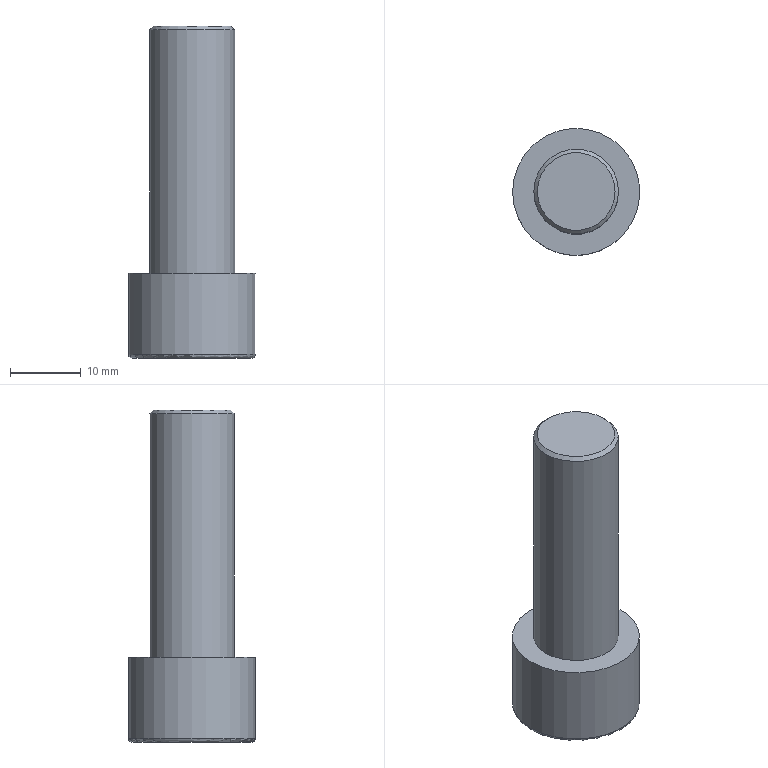Part | NX | features solid 2 | 1 solid | 14 faces | box 18 x 18 x 47 mm | volume 6485 mm3 | plane 10 | cylinder 2 | torus 1 | cone 1 | commonest cylinder face diameters 12 x1 18 x1
STEP:
#1=CARTESIAN_POINT('',(-119.887,-217.,-374.5));
#2=VERTEX_POINT('',#1);
#3=CARTESIAN_POINT('',(-122.774,-212.,-374.5));
#4=VERTEX_POINT('',#3);
#5=CARTESIAN_POINT('',(-119.887,-217.,-374.5));
#6=DIRECTION('',(-0.5,0.866,0.));
#7=VECTOR('',#6,1000.);
#8=LINE('',#5,#7);
#9=EDGE_CURVE('',#2,#4,#8,.T.);
#10=ORIENTED_EDGE('',*,*,#9,.F.);
#11=CARTESIAN_POINT('',(-114.113,-217.,-374.5));
#12=VERTEX_POINT('',#11);
#13=CARTESIAN_POINT('',(-114.113,-217.,-374.5));
#14=DIRECTION('',(-1.,0.,0.));
#15=VECTOR('',#14,1000.);
#16=LINE('',#13,#15);
#17=EDGE_CURVE('',#12,#2,#16,.T.);
#18=ORIENTED_EDGE('',*,*,#17,.F.);
#19=CARTESIAN_POINT('',(-111.226,-212.,-374.5));
#20=VERTEX_POINT('',#19);
#21=CARTESIAN_POINT('',(-111.226,-212.,-374.5));
#22=DIRECTION('',(-0.5,-0.866,0.));
#23=VECTOR('',#22,1000.);
#24=LINE('',#21,#23);
#25=EDGE_CURVE('',#20,#12,#24,.T.);
#26=ORIENTED_EDGE('',*,*,#25,.F.);
#27=CARTESIAN_POINT('',(-114.113,-207.,-374.5));
#28=VERTEX_POINT('',#27);
#29=CARTESIAN_POINT('',(-114.113,-207.,-374.5));
#30=DIRECTION('',(0.5,-0.866,0.));
#31=VECTOR('',#30,1000.);
#32=LINE('',#29,#31);
#33=EDGE_CURVE('',#28,#20,#32,.T.);
#34=ORIENTED_EDGE('',*,*,#33,.F.);
#35=CARTESIAN_POINT('',(-119.887,-207.,-374.5));
#36=VERTEX_POINT('',#35);
#37=CARTESIAN_POINT('',(-119.887,-207.,-374.5));
#38=DIRECTION('',(1.,0.,0.));
#39=VECTOR('',#38,1000.);
#40=LINE('',#37,#39);
#41=EDGE_CURVE('',#36,#28,#40,.T.);
#42=ORIENTED_EDGE('',*,*,#41,.F.);
#43=CARTESIAN_POINT('',(-122.774,-212.,-374.5));
#44=DIRECTION('',(0.5,0.866,0.));
#45=VECTOR('',#44,1000.);
#46=LINE('',#43,#45);
#47=EDGE_CURVE('',#4,#36,#46,.T.);
#48=ORIENTED_EDGE('',*,*,#47,.F.);
#49=EDGE_LOOP('',(#10,#18,#26,#34,#42,#48));
#50=FACE_BOUND('',#49,.T.);
#51=CARTESIAN_POINT('',(-125.5,-212.,-374.5));
#52=VERTEX_POINT('',#51);
#53=CARTESIAN_POINT('',(-117.,-212.,-374.5));
#54=DIRECTION('',(0.,0.,-1.));
#55=DIRECTION('',(-1.,0.,0.));
#56=AXIS2_PLACEMENT_3D('',#53,#54,#55);
#57=CIRCLE('',#56,8.5);
#58=EDGE_CURVE('',#52,#52,#57,.T.);
#59=ORIENTED_EDGE('',*,*,#58,.T.);
#60=EDGE_LOOP('',(#59));
#61=FACE_BOUND('',#60,.T.);
#62=CARTESIAN_POINT('',(-117.,-212.,-374.5));
#63=DIRECTION('',(0.,0.,-1.));
#64=DIRECTION('',(-1.,0.,0.));
#65=AXIS2_PLACEMENT_3D('',#62,#63,#64);
#66=PLANE('',#65);
#67=ADVANCED_FACE('',(#50,#61),#66,.T.);
#68=CARTESIAN_POINT('',(-111.,-212.,-362.5));
#69=VERTEX_POINT('',#68);
#70=CARTESIAN_POINT('',(-117.,-212.,-362.5));
#71=DIRECTION('',(0.,0.,1.));
#72=DIRECTION('',(1.,0.,0.));
#73=AXIS2_PLACEMENT_3D('',#70,#71,#72);
#74=CIRCLE('',#73,6.);
#75=EDGE_CURVE('',#69,#69,#74,.T.);
#76=ORIENTED_EDGE('',*,*,#75,.F.);
#77=EDGE_LOOP('',(#76));
#78=FACE_BOUND('',#77,.T.);
#79=CARTESIAN_POINT('',(-126.,-212.,-362.5));
#80=VERTEX_POINT('',#79);
#81=CARTESIAN_POINT('',(-117.,-212.,-362.5));
#82=DIRECTION('',(0.,0.,-1.));
#83=DIRECTION('',(-1.,0.,0.));
#84=AXIS2_PLACEMENT_3D('',#81,#82,#83);
#85=CIRCLE('',#84,9.);
#86=EDGE_CURVE('',#80,#80,#85,.T.);
#87=ORIENTED_EDGE('',*,*,#86,.F.);
#88=EDGE_LOOP('',(#87));
#89=FACE_BOUND('',#88,.T.);
#90=CARTESIAN_POINT('',(-117.,-212.,-362.5));
#91=DIRECTION('',(0.,0.,1.));
#92=DIRECTION('',(1.,0.,0.));
#93=AXIS2_PLACEMENT_3D('',#90,#91,#92);
#94=PLANE('',#93);
#95=ADVANCED_FACE('',(#78,#89),#94,.T.);
#96=CARTESIAN_POINT('',(-126.,-212.,-374.));
#97=VERTEX_POINT('',#96);
#98=CARTESIAN_POINT('',(-117.,-212.,-374.));
#99=DIRECTION('',(0.,0.,-1.));
#100=DIRECTION('',(-1.,0.,0.));
#101=AXIS2_PLACEMENT_3D('',#98,#99,#100);
#102=CIRCLE('',#101,9.);
#103=EDGE_CURVE('',#97,#97,#102,.F.);
#104=ORIENTED_EDGE('',*,*,#103,.T.);
#105=EDGE_LOOP('',(#104));
#106=FACE_BOUND('',#105,.T.);
#107=ORIENTED_EDGE('',*,*,#86,.T.);
#108=EDGE_LOOP('',(#107));
#109=FACE_BOUND('',#108,.T.);
#110=CARTESIAN_POINT('',(-117.,-212.,-362.5));
#111=DIRECTION('',(0.,0.,-1.));
#112=DIRECTION('',(-1.,0.,0.));
#113=AXIS2_PLACEMENT_3D('',#110,#111,#112);
#114=CYLINDRICAL_SURFACE('',#113,9.);
#115=ADVANCED_FACE('',(#106,#109),#114,.T.);
#116=ORIENTED_EDGE('',*,*,#58,.F.);
#117=EDGE_LOOP('',(#116));
#118=FACE_BOUND('',#117,.T.);
#119=ORIENTED_EDGE('',*,*,#103,.F.);
#120=EDGE_LOOP('',(#119));
#121=FACE_BOUND('',#120,.T.);
#122=CARTESIAN_POINT('',(-117.,-212.,-374.));
#123=DIRECTION('',(0.,0.,-1.));
#124=DIRECTION('',(-1.,0.,0.));
#125=AXIS2_PLACEMENT_3D('',#122,#123,#124);
#126=TOROIDAL_SURFACE('',#125,8.5,0.5);
#127=ADVANCED_FACE('',(#118,#121),#126,.T.);
#128=CARTESIAN_POINT('',(-111.5,-212.,-327.5));
#129=VERTEX_POINT('',#128);
#130=CARTESIAN_POINT('',(-117.,-212.,-327.5));
#131=DIRECTION('',(0.,0.,1.));
#132=DIRECTION('',(1.,0.,0.));
#133=AXIS2_PLACEMENT_3D('',#130,#131,#132);
#134=CIRCLE('',#133,5.5);
#135=EDGE_CURVE('',#129,#129,#134,.T.);
#136=ORIENTED_EDGE('',*,*,#135,.T.);
#137=EDGE_LOOP('',(#136));
#138=FACE_BOUND('',#137,.T.);
#139=CARTESIAN_POINT('',(-117.,-212.,-327.5));
#140=DIRECTION('',(0.,0.,1.));
#141=DIRECTION('',(1.,0.,0.));
#142=AXIS2_PLACEMENT_3D('',#139,#140,#141);
#143=PLANE('',#142);
#144=ADVANCED_FACE('',(#138),#143,.T.);
#145=CARTESIAN_POINT('',(-111.,-212.,-328.));
#146=VERTEX_POINT('',#145);
#147=CARTESIAN_POINT('',(-117.,-212.,-328.));
#148=DIRECTION('',(0.,0.,1.));
#149=DIRECTION('',(1.,0.,0.));
#150=AXIS2_PLACEMENT_3D('',#147,#148,#149);
#151=CIRCLE('',#150,6.);
#152=EDGE_CURVE('',#146,#146,#151,.F.);
#153=ORIENTED_EDGE('',*,*,#152,.T.);
#154=EDGE_LOOP('',(#153));
#155=FACE_BOUND('',#154,.T.);
#156=ORIENTED_EDGE('',*,*,#75,.T.);
#157=EDGE_LOOP('',(#156));
#158=FACE_BOUND('',#157,.T.);
#159=CARTESIAN_POINT('',(-117.,-212.,-327.5));
#160=DIRECTION('',(0.,0.,-1.));
#161=DIRECTION('',(-1.,0.,0.));
#162=AXIS2_PLACEMENT_3D('',#159,#160,#161);
#163=CYLINDRICAL_SURFACE('',#162,6.);
#164=ADVANCED_FACE('',(#155,#158),#163,.T.);
#165=ORIENTED_EDGE('',*,*,#135,.F.);
#166=EDGE_LOOP('',(#165));
#167=FACE_BOUND('',#166,.T.);
#168=ORIENTED_EDGE('',*,*,#152,.F.);
#169=EDGE_LOOP('',(#168));
#170=FACE_BOUND('',#169,.T.);
#171=CARTESIAN_POINT('',(-117.,-212.,-328.));
#172=DIRECTION('',(0.,0.,-1.));
#173=DIRECTION('',(-1.,0.,0.));
#174=AXIS2_PLACEMENT_3D('',#171,#172,#173);
#175=CONICAL_SURFACE('',#174,6.,0.7854);
#176=ADVANCED_FACE('',(#167,#170),#175,.T.);
#177=ORIENTED_EDGE('',*,*,#9,.T.);
#178=CARTESIAN_POINT('',(-122.774,-212.,-368.5));
#179=VERTEX_POINT('',#178);
#180=CARTESIAN_POINT('',(-122.774,-212.,-368.5));
#181=DIRECTION('',(0.,0.,-1.));
#182=VECTOR('',#181,1000.);
#183=LINE('',#180,#182);
#184=EDGE_CURVE('',#179,#4,#183,.T.);
#185=ORIENTED_EDGE('',*,*,#184,.F.);
#186=CARTESIAN_POINT('',(-119.887,-217.,-368.5));
#187=VERTEX_POINT('',#186);
#188=CARTESIAN_POINT('',(-119.887,-217.,-368.5));
#189=DIRECTION('',(-0.5,0.866,0.));
#190=VECTOR('',#189,1000.);
#191=LINE('',#188,#190);
#192=EDGE_CURVE('',#187,#179,#191,.T.);
#193=ORIENTED_EDGE('',*,*,#192,.F.);
#194=CARTESIAN_POINT('',(-119.887,-217.,-368.5));
#195=DIRECTION('',(0.,0.,-1.));
#196=VECTOR('',#195,1000.);
#197=LINE('',#194,#196);
#198=EDGE_CURVE('',#187,#2,#197,.T.);
#199=ORIENTED_EDGE('',*,*,#198,.T.);
#200=EDGE_LOOP('',(#177,#185,#193,#199));
#201=FACE_BOUND('',#200,.T.);
#202=CARTESIAN_POINT('',(-121.33,-214.5,-371.5));
#203=DIRECTION('',(-0.866,-0.5,0.));
#204=DIRECTION('',(0.5,-0.866,0.));
#205=AXIS2_PLACEMENT_3D('',#202,#203,#204);
#206=PLANE('',#205);
#207=ADVANCED_FACE('',(#201),#206,.F.);
#208=ORIENTED_EDGE('',*,*,#17,.T.);
#209=ORIENTED_EDGE('',*,*,#198,.F.);
#210=CARTESIAN_POINT('',(-114.113,-217.,-368.5));
#211=VERTEX_POINT('',#210);
#212=CARTESIAN_POINT('',(-114.113,-217.,-368.5));
#213=DIRECTION('',(-1.,0.,0.));
#214=VECTOR('',#213,1000.);
#215=LINE('',#212,#214);
#216=EDGE_CURVE('',#211,#187,#215,.T.);
#217=ORIENTED_EDGE('',*,*,#216,.F.);
#218=CARTESIAN_POINT('',(-114.113,-217.,-368.5));
#219=DIRECTION('',(0.,0.,-1.));
#220=VECTOR('',#219,1000.);
#221=LINE('',#218,#220);
#222=EDGE_CURVE('',#211,#12,#221,.T.);
#223=ORIENTED_EDGE('',*,*,#222,.T.);
#224=EDGE_LOOP('',(#208,#209,#217,#223));
#225=FACE_BOUND('',#224,.T.);
#226=CARTESIAN_POINT('',(-117.,-217.,-371.5));
#227=DIRECTION('',(0.,-1.,0.));
#228=DIRECTION('',(1.,0.,0.));
#229=AXIS2_PLACEMENT_3D('',#226,#227,#228);
#230=PLANE('',#229);
#231=ADVANCED_FACE('',(#225),#230,.F.);
#232=ORIENTED_EDGE('',*,*,#25,.T.);
#233=ORIENTED_EDGE('',*,*,#222,.F.);
#234=CARTESIAN_POINT('',(-111.226,-212.,-368.5));
#235=VERTEX_POINT('',#234);
#236=CARTESIAN_POINT('',(-111.226,-212.,-368.5));
#237=DIRECTION('',(-0.5,-0.866,0.));
#238=VECTOR('',#237,1000.);
#239=LINE('',#236,#238);
#240=EDGE_CURVE('',#235,#211,#239,.T.);
#241=ORIENTED_EDGE('',*,*,#240,.F.);
#242=CARTESIAN_POINT('',(-111.226,-212.,-368.5));
#243=DIRECTION('',(0.,0.,-1.));
#244=VECTOR('',#243,1000.);
#245=LINE('',#242,#244);
#246=EDGE_CURVE('',#235,#20,#245,.T.);
#247=ORIENTED_EDGE('',*,*,#246,.T.);
#248=EDGE_LOOP('',(#232,#233,#241,#247));
#249=FACE_BOUND('',#248,.T.);
#250=CARTESIAN_POINT('',(-112.67,-214.5,-371.5));
#251=DIRECTION('',(0.866,-0.5,0.));
#252=DIRECTION('',(0.5,0.866,0.));
#253=AXIS2_PLACEMENT_3D('',#250,#251,#252);
#254=PLANE('',#253);
#255=ADVANCED_FACE('',(#249),#254,.F.);
#256=ORIENTED_EDGE('',*,*,#33,.T.);
#257=ORIENTED_EDGE('',*,*,#246,.F.);
#258=CARTESIAN_POINT('',(-114.113,-207.,-368.5));
#259=VERTEX_POINT('',#258);
#260=CARTESIAN_POINT('',(-114.113,-207.,-368.5));
#261=DIRECTION('',(0.5,-0.866,0.));
#262=VECTOR('',#261,1000.);
#263=LINE('',#260,#262);
#264=EDGE_CURVE('',#259,#235,#263,.T.);
#265=ORIENTED_EDGE('',*,*,#264,.F.);
#266=CARTESIAN_POINT('',(-114.113,-207.,-368.5));
#267=DIRECTION('',(0.,0.,-1.));
#268=VECTOR('',#267,1000.);
#269=LINE('',#266,#268);
#270=EDGE_CURVE('',#259,#28,#269,.T.);
#271=ORIENTED_EDGE('',*,*,#270,.T.);
#272=EDGE_LOOP('',(#256,#257,#265,#271));
#273=FACE_BOUND('',#272,.T.);
#274=CARTESIAN_POINT('',(-112.67,-209.5,-371.5));
#275=DIRECTION('',(0.866,0.5,0.));
#276=DIRECTION('',(-0.5,0.866,0.));
#277=AXIS2_PLACEMENT_3D('',#274,#275,#276);
#278=PLANE('',#277);
#279=ADVANCED_FACE('',(#273),#278,.F.);
#280=ORIENTED_EDGE('',*,*,#41,.T.);
#281=ORIENTED_EDGE('',*,*,#270,.F.);
#282=CARTESIAN_POINT('',(-119.887,-207.,-368.5));
#283=VERTEX_POINT('',#282);
#284=CARTESIAN_POINT('',(-119.887,-207.,-368.5));
#285=DIRECTION('',(1.,0.,0.));
#286=VECTOR('',#285,1000.);
#287=LINE('',#284,#286);
#288=EDGE_CURVE('',#283,#259,#287,.T.);
#289=ORIENTED_EDGE('',*,*,#288,.F.);
#290=CARTESIAN_POINT('',(-119.887,-207.,-368.5));
#291=DIRECTION('',(0.,0.,-1.));
#292=VECTOR('',#291,1000.);
#293=LINE('',#290,#292);
#294=EDGE_CURVE('',#283,#36,#293,.T.);
#295=ORIENTED_EDGE('',*,*,#294,.T.);
#296=EDGE_LOOP('',(#280,#281,#289,#295));
#297=FACE_BOUND('',#296,.T.);
#298=CARTESIAN_POINT('',(-117.,-207.,-371.5));
#299=DIRECTION('',(0.,1.,0.));
#300=DIRECTION('',(0.,0.,1.));
#301=AXIS2_PLACEMENT_3D('',#298,#299,#300);
#302=PLANE('',#301);
#303=ADVANCED_FACE('',(#297),#302,.F.);
#304=ORIENTED_EDGE('',*,*,#47,.T.);
#305=ORIENTED_EDGE('',*,*,#294,.F.);
#306=CARTESIAN_POINT('',(-122.774,-212.,-368.5));
#307=DIRECTION('',(0.5,0.866,0.));
#308=VECTOR('',#307,1000.);
#309=LINE('',#306,#308);
#310=EDGE_CURVE('',#179,#283,#309,.T.);
#311=ORIENTED_EDGE('',*,*,#310,.F.);
#312=ORIENTED_EDGE('',*,*,#184,.T.);
#313=EDGE_LOOP('',(#304,#305,#311,#312));
#314=FACE_BOUND('',#313,.T.);
#315=CARTESIAN_POINT('',(-121.33,-209.5,-371.5));
#316=DIRECTION('',(-0.866,0.5,0.));
#317=DIRECTION('',(-0.5,-0.866,0.));
#318=AXIS2_PLACEMENT_3D('',#315,#316,#317);
#319=PLANE('',#318);
#320=ADVANCED_FACE('',(#314),#319,.F.);
#321=ORIENTED_EDGE('',*,*,#310,.T.);
#322=ORIENTED_EDGE('',*,*,#288,.T.);
#323=ORIENTED_EDGE('',*,*,#264,.T.);
#324=ORIENTED_EDGE('',*,*,#240,.T.);
#325=ORIENTED_EDGE('',*,*,#216,.T.);
#326=ORIENTED_EDGE('',*,*,#192,.T.);
#327=EDGE_LOOP('',(#321,#322,#323,#324,#325,#326));
#328=FACE_BOUND('',#327,.T.);
#329=CARTESIAN_POINT('',(-117.,-212.,-368.5));
#330=DIRECTION('',(0.,0.,1.));
#331=DIRECTION('',(1.,0.,0.));
#332=AXIS2_PLACEMENT_3D('',#329,#330,#331);
#333=PLANE('',#332);
#334=ADVANCED_FACE('',(#328),#333,.F.);
#335=CLOSED_SHELL('',(#67,#95,#115,#127,#144,#164,#176,#207,#231,#255,#279,#303,#320,#334));
#336=MANIFOLD_SOLID_BREP('',#335);
#337=(LENGTH_UNIT()NAMED_UNIT(*)SI_UNIT(.MILLI.,.METRE.));
#338=UNCERTAINTY_MEASURE_WITH_UNIT(LENGTH_MEASURE(0.00001),#337,'','');
#339=(NAMED_UNIT(*)PLANE_ANGLE_UNIT()SI_UNIT($,.RADIAN.));
#340=(NAMED_UNIT(*)SI_UNIT($,.STERADIAN.)SOLID_ANGLE_UNIT());
#341=(GEOMETRIC_REPRESENTATION_CONTEXT(3)GLOBAL_UNCERTAINTY_ASSIGNED_CONTEXT((#338))GLOBAL_UNIT_ASSIGNED_CONTEXT((#337,#339,#340))REPRESENTATION_CONTEXT('',''));
#342=ADVANCED_BREP_SHAPE_REPRESENTATION('',(#336),#341);